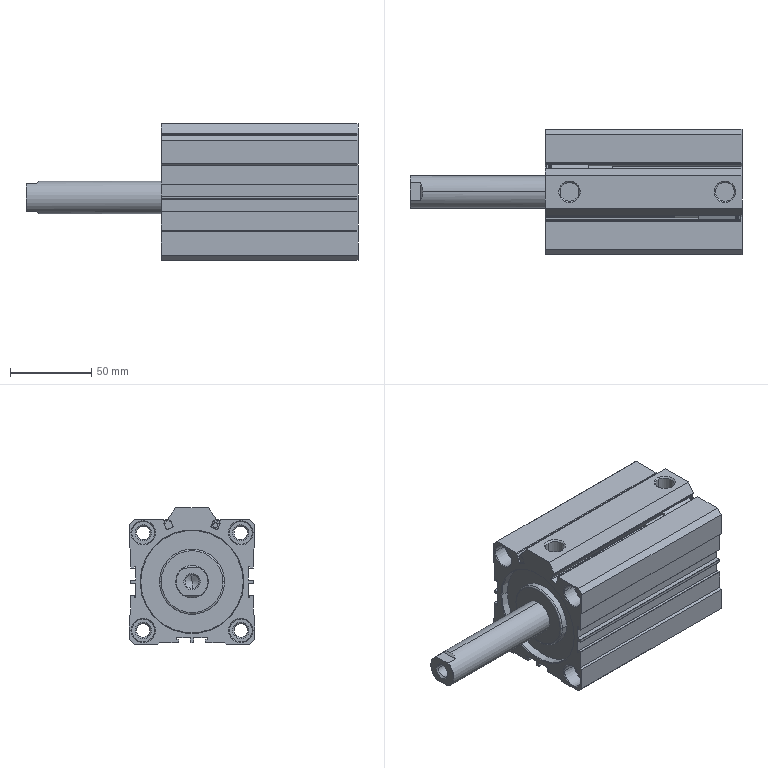Part | SolidWorks | 4 solids | 312 faces | box 204 x 77 x 84 mm | volume 434745 mm3 | plane 130 | cylinder 118 | cone 62 | spline 2 | commonest cylinder face diameters 0.4 x39 14 x16 0.8 x15 8.376 x10 63 x6 0.6 x4